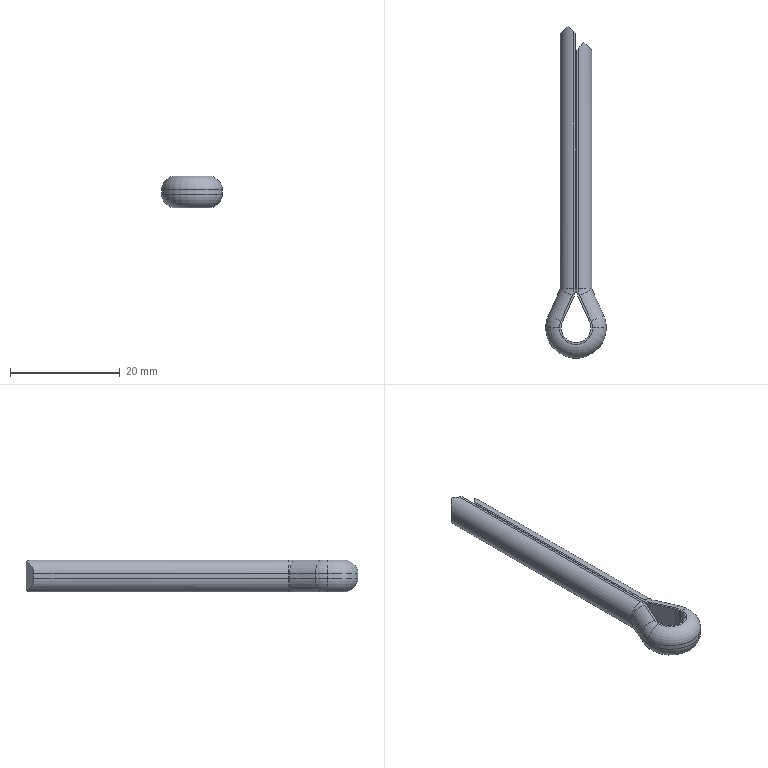Part | STEP file | SLIDER_SHAFT1V11 | 1 solid | 42 faces | box 11.05 x 60.6 x 5.8 mm | volume 1645 mm3 | cylinder 18 | plane 14 | torus 10 | commonest cylinder face diameters 5 x8 5.366 x3 11.05 x3 1.16 x2 6.844 x2